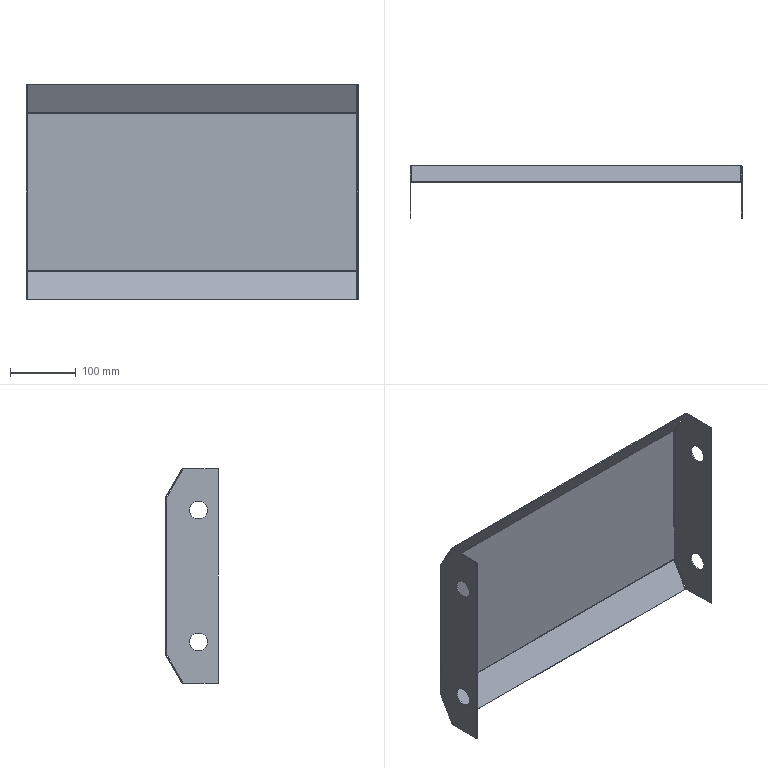Part | STEP file | 1 solid | 50 faces | box 504 x 80 x 327.138 mm | volume 217529 mm3 | plane 34 | cylinder 16 | commonest cylinder face diameters 27 x8 2 x4 4 x4